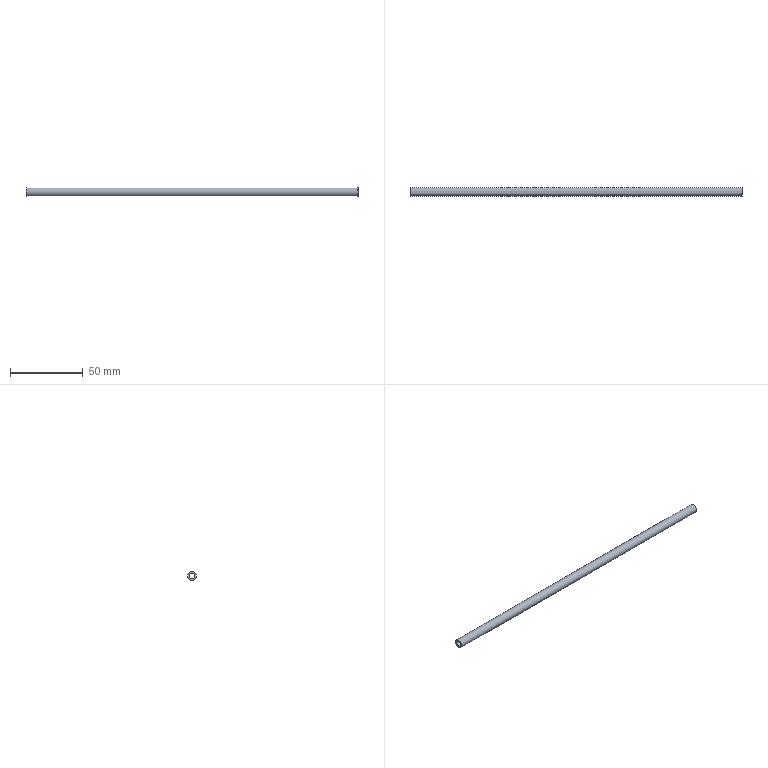Part | NX | features solid 2 | 1 solid | 4 faces | box 228.824 x 6 x 6 mm | volume 3594 mm3 | cylinder 2 | plane 2 | commonest cylinder face diameters 4 x1 6 x1
STEP:
#1=CARTESIAN_POINT('',(-323.824,-64.,347.));
#2=VERTEX_POINT('',#1);
#3=CARTESIAN_POINT('',(-323.824,-62.,347.));
#4=DIRECTION('',(-1.,0.,0.));
#5=DIRECTION('',(0.,-1.,0.));
#6=AXIS2_PLACEMENT_3D('',#3,#4,#5);
#7=CIRCLE('',#6,2.);
#8=EDGE_CURVE('',#2,#2,#7,.T.);
#9=ORIENTED_EDGE('',*,*,#8,.T.);
#10=EDGE_LOOP('',(#9));
#11=FACE_BOUND('',#10,.T.);
#12=CARTESIAN_POINT('',(-95.,-64.,347.));
#13=VERTEX_POINT('',#12);
#14=CARTESIAN_POINT('',(-95.,-62.,347.));
#15=DIRECTION('',(-1.,0.,0.));
#16=DIRECTION('',(0.,-1.,0.));
#17=AXIS2_PLACEMENT_3D('',#14,#15,#16);
#18=CIRCLE('',#17,2.);
#19=EDGE_CURVE('',#13,#13,#18,.T.);
#20=ORIENTED_EDGE('',*,*,#19,.F.);
#21=EDGE_LOOP('',(#20));
#22=FACE_BOUND('',#21,.T.);
#23=CARTESIAN_POINT('',(-273.824,-62.,347.));
#24=DIRECTION('',(1.,0.,0.));
#25=DIRECTION('',(0.,1.,0.));
#26=AXIS2_PLACEMENT_3D('',#23,#24,#25);
#27=CYLINDRICAL_SURFACE('',#26,2.);
#28=ADVANCED_FACE('',(#11,#22),#27,.F.);
#29=CARTESIAN_POINT('',(-323.824,-65.,347.));
#30=VERTEX_POINT('',#29);
#31=CARTESIAN_POINT('',(-323.824,-62.,347.));
#32=DIRECTION('',(-1.,0.,0.));
#33=DIRECTION('',(0.,-1.,0.));
#34=AXIS2_PLACEMENT_3D('',#31,#32,#33);
#35=CIRCLE('',#34,3.);
#36=EDGE_CURVE('',#30,#30,#35,.T.);
#37=ORIENTED_EDGE('',*,*,#36,.F.);
#38=EDGE_LOOP('',(#37));
#39=FACE_BOUND('',#38,.T.);
#40=CARTESIAN_POINT('',(-95.,-65.,347.));
#41=VERTEX_POINT('',#40);
#42=CARTESIAN_POINT('',(-95.,-62.,347.));
#43=DIRECTION('',(-1.,0.,0.));
#44=DIRECTION('',(0.,-1.,0.));
#45=AXIS2_PLACEMENT_3D('',#42,#43,#44);
#46=CIRCLE('',#45,3.);
#47=EDGE_CURVE('',#41,#41,#46,.T.);
#48=ORIENTED_EDGE('',*,*,#47,.T.);
#49=EDGE_LOOP('',(#48));
#50=FACE_BOUND('',#49,.T.);
#51=CARTESIAN_POINT('',(-273.824,-62.,347.));
#52=DIRECTION('',(1.,0.,0.));
#53=DIRECTION('',(0.,1.,0.));
#54=AXIS2_PLACEMENT_3D('',#51,#52,#53);
#55=CYLINDRICAL_SURFACE('',#54,3.);
#56=ADVANCED_FACE('',(#39,#50),#55,.T.);
#57=ORIENTED_EDGE('',*,*,#8,.F.);
#58=EDGE_LOOP('',(#57));
#59=FACE_BOUND('',#58,.T.);
#60=ORIENTED_EDGE('',*,*,#36,.T.);
#61=EDGE_LOOP('',(#60));
#62=FACE_BOUND('',#61,.T.);
#63=CARTESIAN_POINT('',(-323.824,-62.,347.));
#64=DIRECTION('',(-1.,0.,0.));
#65=DIRECTION('',(0.,-1.,0.));
#66=AXIS2_PLACEMENT_3D('',#63,#64,#65);
#67=PLANE('',#66);
#68=ADVANCED_FACE('',(#59,#62),#67,.T.);
#69=ORIENTED_EDGE('',*,*,#19,.T.);
#70=EDGE_LOOP('',(#69));
#71=FACE_BOUND('',#70,.T.);
#72=ORIENTED_EDGE('',*,*,#47,.F.);
#73=EDGE_LOOP('',(#72));
#74=FACE_BOUND('',#73,.T.);
#75=CARTESIAN_POINT('',(-95.,-62.,347.));
#76=DIRECTION('',(-1.,0.,0.));
#77=DIRECTION('',(0.,-1.,0.));
#78=AXIS2_PLACEMENT_3D('',#75,#76,#77);
#79=PLANE('',#78);
#80=ADVANCED_FACE('',(#71,#74),#79,.F.);
#81=CLOSED_SHELL('',(#28,#56,#68,#80));
#82=MANIFOLD_SOLID_BREP('',#81);
#83=(LENGTH_UNIT()NAMED_UNIT(*)SI_UNIT(.MILLI.,.METRE.));
#84=UNCERTAINTY_MEASURE_WITH_UNIT(LENGTH_MEASURE(0.00001),#83,'','');
#85=(NAMED_UNIT(*)PLANE_ANGLE_UNIT()SI_UNIT($,.RADIAN.));
#86=(NAMED_UNIT(*)SI_UNIT($,.STERADIAN.)SOLID_ANGLE_UNIT());
#87=(GEOMETRIC_REPRESENTATION_CONTEXT(3)GLOBAL_UNCERTAINTY_ASSIGNED_CONTEXT((#84))GLOBAL_UNIT_ASSIGNED_CONTEXT((#83,#85,#86))REPRESENTATION_CONTEXT('',''));
#88=ADVANCED_BREP_SHAPE_REPRESENTATION('',(#82),#87);